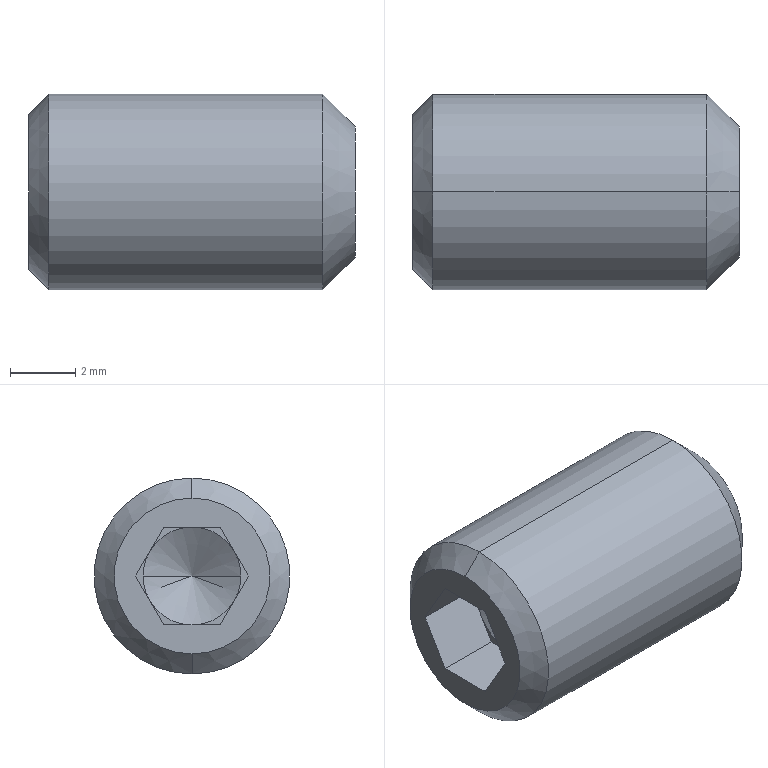Part | SolidWorks | features BaseBody 1 | 1 solid | 22 faces | box 10 x 6 x 6 mm | volume 253.469 mm3 | plane 14 | cone 6 | cylinder 2 | commonest cylinder face diameters 6 x2
STEP:
#1=CARTESIAN_POINT('',(4.,0.,3.));
#2=VERTEX_POINT('',#1);
#3=CARTESIAN_POINT('',(4.,0.,-3.));
#4=VERTEX_POINT('',#3);
#5=CARTESIAN_POINT('',(4.,0.,0.));
#6=DIRECTION('',(-1.,0.,0.));
#7=DIRECTION('',(0.,0.,1.));
#8=AXIS2_PLACEMENT_3D('',#5,#6,#7);
#9=CIRCLE('',#8,3.);
#10=EDGE_CURVE('',#2,#4,#9,.T.);
#11=ORIENTED_EDGE('',*,*,#10,.T.);
#12=CARTESIAN_POINT('',(-4.387,0.,-3.));
#13=VERTEX_POINT('',#12);
#14=CARTESIAN_POINT('',(5.,0.,-3.));
#15=DIRECTION('',(-1.,0.,0.));
#16=VECTOR('',#15,1000.);
#17=LINE('',#14,#16);
#18=EDGE_CURVE('',#4,#13,#17,.T.);
#19=ORIENTED_EDGE('',*,*,#18,.T.);
#20=CARTESIAN_POINT('',(-4.387,0.,3.));
#21=VERTEX_POINT('',#20);
#22=CARTESIAN_POINT('',(-4.387,0.,0.));
#23=DIRECTION('',(1.,0.,0.));
#24=DIRECTION('',(0.,0.,1.));
#25=AXIS2_PLACEMENT_3D('',#22,#23,#24);
#26=CIRCLE('',#25,3.);
#27=EDGE_CURVE('',#13,#21,#26,.T.);
#28=ORIENTED_EDGE('',*,*,#27,.T.);
#29=CARTESIAN_POINT('',(5.,0.,3.));
#30=DIRECTION('',(-1.,0.,0.));
#31=VECTOR('',#30,1000.);
#32=LINE('',#29,#31);
#33=EDGE_CURVE('',#2,#21,#32,.T.);
#34=ORIENTED_EDGE('',*,*,#33,.F.);
#35=EDGE_LOOP('',(#11,#19,#28,#34));
#36=FACE_OUTER_BOUND('',#35,.T.);
#37=CARTESIAN_POINT('',(5.,0.,0.));
#38=DIRECTION('',(-1.,0.,0.));
#39=DIRECTION('',(0.,0.,1.));
#40=AXIS2_PLACEMENT_3D('',#37,#38,#39);
#41=CYLINDRICAL_SURFACE('',#40,3.);
#42=ADVANCED_FACE('',(#36),#41,.T.);
#43=CARTESIAN_POINT('',(-5.,0.,-2.387));
#44=VERTEX_POINT('',#43);
#45=CARTESIAN_POINT('',(-5.,0.,2.387));
#46=VERTEX_POINT('',#45);
#47=CARTESIAN_POINT('',(-5.,0.,0.));
#48=DIRECTION('',(1.,0.,0.));
#49=DIRECTION('',(0.,0.,-1.));
#50=AXIS2_PLACEMENT_3D('',#47,#48,#49);
#51=CIRCLE('',#50,2.387);
#52=EDGE_CURVE('',#44,#46,#51,.T.);
#53=ORIENTED_EDGE('',*,*,#52,.T.);
#54=CARTESIAN_POINT('',(-4.387,0.,3.));
#55=DIRECTION('',(0.7071,0.,0.7071));
#56=VECTOR('',#55,1000.);
#57=LINE('',#54,#56);
#58=EDGE_CURVE('',#46,#21,#57,.T.);
#59=ORIENTED_EDGE('',*,*,#58,.T.);
#60=ORIENTED_EDGE('',*,*,#27,.F.);
#61=CARTESIAN_POINT('',(-4.387,0.,-3.));
#62=DIRECTION('',(0.7071,0.,-0.7071));
#63=VECTOR('',#62,1000.);
#64=LINE('',#61,#63);
#65=EDGE_CURVE('',#44,#13,#64,.T.);
#66=ORIENTED_EDGE('',*,*,#65,.F.);
#67=EDGE_LOOP('',(#53,#59,#60,#66));
#68=FACE_OUTER_BOUND('',#67,.T.);
#69=CARTESIAN_POINT('',(-4.387,0.,0.));
#70=DIRECTION('',(1.,0.,0.));
#71=DIRECTION('',(0.,0.,-1.));
#72=AXIS2_PLACEMENT_3D('',#69,#70,#71);
#73=CONICAL_SURFACE('',#72,3.,0.7854);
#74=ADVANCED_FACE('',(#68),#73,.T.);
#75=CARTESIAN_POINT('',(5.,0.,2.));
#76=VERTEX_POINT('',#75);
#77=CARTESIAN_POINT('',(5.,0.,-2.));
#78=VERTEX_POINT('',#77);
#79=CARTESIAN_POINT('',(5.,0.,0.));
#80=DIRECTION('',(-1.,0.,0.));
#81=DIRECTION('',(0.,0.,1.));
#82=AXIS2_PLACEMENT_3D('',#79,#80,#81);
#83=CIRCLE('',#82,2.);
#84=EDGE_CURVE('',#76,#78,#83,.T.);
#85=ORIENTED_EDGE('',*,*,#84,.T.);
#86=CARTESIAN_POINT('',(4.,0.,-3.));
#87=DIRECTION('',(-0.7071,0.,-0.7071));
#88=VECTOR('',#87,1000.);
#89=LINE('',#86,#88);
#90=EDGE_CURVE('',#78,#4,#89,.T.);
#91=ORIENTED_EDGE('',*,*,#90,.T.);
#92=ORIENTED_EDGE('',*,*,#10,.F.);
#93=CARTESIAN_POINT('',(4.,0.,3.));
#94=DIRECTION('',(-0.7071,0.,0.7071));
#95=VECTOR('',#94,1000.);
#96=LINE('',#93,#95);
#97=EDGE_CURVE('',#76,#2,#96,.T.);
#98=ORIENTED_EDGE('',*,*,#97,.F.);
#99=EDGE_LOOP('',(#85,#91,#92,#98));
#100=FACE_OUTER_BOUND('',#99,.T.);
#101=CARTESIAN_POINT('',(4.,0.,0.));
#102=DIRECTION('',(-1.,0.,0.));
#103=DIRECTION('',(0.,0.,1.));
#104=AXIS2_PLACEMENT_3D('',#101,#102,#103);
#105=CONICAL_SURFACE('',#104,3.,0.7854);
#106=ADVANCED_FACE('',(#100),#105,.T.);
#107=CARTESIAN_POINT('',(-2.15,0.,0.));
#108=VERTEX_POINT('',#107);
#109=CARTESIAN_POINT('',(-3.,-1.5,0.));
#110=VERTEX_POINT('',#109);
#111=CARTESIAN_POINT('',(-3.,-1.5,0.));
#112=DIRECTION('',(-0.493,-0.87,0.));
#113=VECTOR('',#112,1000.);
#114=LINE('',#111,#113);
#115=EDGE_CURVE('',#108,#110,#114,.T.);
#116=ORIENTED_EDGE('',*,*,#115,.F.);
#117=CARTESIAN_POINT('',(-3.,1.5,0.));
#118=VERTEX_POINT('',#117);
#119=CARTESIAN_POINT('',(-3.,1.5,0.));
#120=DIRECTION('',(-0.493,0.87,0.));
#121=VECTOR('',#120,1000.);
#122=LINE('',#119,#121);
#123=EDGE_CURVE('',#108,#118,#122,.T.);
#124=ORIENTED_EDGE('',*,*,#123,.T.);
#125=CARTESIAN_POINT('',(-3.,1.299,-0.75));
#126=VERTEX_POINT('',#125);
#127=CARTESIAN_POINT('',(-3.,0.,0.));
#128=DIRECTION('',(-1.,0.,0.));
#129=DIRECTION('',(0.,-1.,0.));
#130=AXIS2_PLACEMENT_3D('',#127,#128,#129);
#131=CIRCLE('',#130,1.5);
#132=EDGE_CURVE('',#118,#126,#131,.T.);
#133=ORIENTED_EDGE('',*,*,#132,.T.);
#134=CARTESIAN_POINT('',(-3.,0.,-1.5));
#135=VERTEX_POINT('',#134);
#136=CARTESIAN_POINT('',(-3.,0.,0.));
#137=DIRECTION('',(1.,0.,0.));
#138=DIRECTION('',(0.,-1.,0.));
#139=AXIS2_PLACEMENT_3D('',#136,#137,#138);
#140=CIRCLE('',#139,1.5);
#141=EDGE_CURVE('',#135,#126,#140,.T.);
#142=ORIENTED_EDGE('',*,*,#141,.F.);
#143=CARTESIAN_POINT('',(-3.,-1.299,-0.75));
#144=VERTEX_POINT('',#143);
#145=CARTESIAN_POINT('',(-3.,0.,0.));
#146=DIRECTION('',(1.,0.,0.));
#147=DIRECTION('',(0.,-1.,0.));
#148=AXIS2_PLACEMENT_3D('',#145,#146,#147);
#149=CIRCLE('',#148,1.5);
#150=EDGE_CURVE('',#144,#135,#149,.T.);
#151=ORIENTED_EDGE('',*,*,#150,.F.);
#152=CARTESIAN_POINT('',(-3.,0.,0.));
#153=DIRECTION('',(1.,0.,0.));
#154=DIRECTION('',(0.,-1.,0.));
#155=AXIS2_PLACEMENT_3D('',#152,#153,#154);
#156=CIRCLE('',#155,1.5);
#157=EDGE_CURVE('',#110,#144,#156,.T.);
#158=ORIENTED_EDGE('',*,*,#157,.F.);
#159=EDGE_LOOP('',(#116,#124,#133,#142,#151,#158));
#160=FACE_OUTER_BOUND('',#159,.T.);
#161=CARTESIAN_POINT('',(-3.,0.,0.));
#162=DIRECTION('',(-1.,0.,0.));
#163=DIRECTION('',(0.,-1.,0.));
#164=AXIS2_PLACEMENT_3D('',#161,#162,#163);
#165=CONICAL_SURFACE('',#164,1.5,1.055);
#166=ADVANCED_FACE('',(#160),#165,.F.);
#167=ORIENTED_EDGE('',*,*,#18,.F.);
#168=CARTESIAN_POINT('',(4.,0.,0.));
#169=DIRECTION('',(-1.,0.,0.));
#170=DIRECTION('',(0.,0.,1.));
#171=AXIS2_PLACEMENT_3D('',#168,#169,#170);
#172=CIRCLE('',#171,3.);
#173=EDGE_CURVE('',#4,#2,#172,.T.);
#174=ORIENTED_EDGE('',*,*,#173,.T.);
#175=ORIENTED_EDGE('',*,*,#33,.T.);
#176=CARTESIAN_POINT('',(-4.387,0.,0.));
#177=DIRECTION('',(1.,0.,0.));
#178=DIRECTION('',(0.,0.,1.));
#179=AXIS2_PLACEMENT_3D('',#176,#177,#178);
#180=CIRCLE('',#179,3.);
#181=EDGE_CURVE('',#21,#13,#180,.T.);
#182=ORIENTED_EDGE('',*,*,#181,.T.);
#183=EDGE_LOOP('',(#167,#174,#175,#182));
#184=FACE_OUTER_BOUND('',#183,.T.);
#185=CARTESIAN_POINT('',(5.,0.,0.));
#186=DIRECTION('',(-1.,0.,0.));
#187=DIRECTION('',(0.,0.,1.));
#188=AXIS2_PLACEMENT_3D('',#185,#186,#187);
#189=CYLINDRICAL_SURFACE('',#188,3.);
#190=ADVANCED_FACE('',(#184),#189,.T.);
#191=ORIENTED_EDGE('',*,*,#58,.F.);
#192=CARTESIAN_POINT('',(-5.,0.,0.));
#193=DIRECTION('',(1.,0.,0.));
#194=DIRECTION('',(0.,0.,-1.));
#195=AXIS2_PLACEMENT_3D('',#192,#193,#194);
#196=CIRCLE('',#195,2.387);
#197=EDGE_CURVE('',#46,#44,#196,.T.);
#198=ORIENTED_EDGE('',*,*,#197,.T.);
#199=ORIENTED_EDGE('',*,*,#65,.T.);
#200=ORIENTED_EDGE('',*,*,#181,.F.);
#201=EDGE_LOOP('',(#191,#198,#199,#200));
#202=FACE_OUTER_BOUND('',#201,.T.);
#203=CARTESIAN_POINT('',(-4.387,0.,0.));
#204=DIRECTION('',(1.,0.,0.));
#205=DIRECTION('',(0.,0.,-1.));
#206=AXIS2_PLACEMENT_3D('',#203,#204,#205);
#207=CONICAL_SURFACE('',#206,3.,0.7854);
#208=ADVANCED_FACE('',(#202),#207,.T.);
#209=ORIENTED_EDGE('',*,*,#90,.F.);
#210=CARTESIAN_POINT('',(5.,0.,0.));
#211=DIRECTION('',(-1.,0.,0.));
#212=DIRECTION('',(0.,0.,1.));
#213=AXIS2_PLACEMENT_3D('',#210,#211,#212);
#214=CIRCLE('',#213,2.);
#215=EDGE_CURVE('',#78,#76,#214,.T.);
#216=ORIENTED_EDGE('',*,*,#215,.T.);
#217=ORIENTED_EDGE('',*,*,#97,.T.);
#218=ORIENTED_EDGE('',*,*,#173,.F.);
#219=EDGE_LOOP('',(#209,#216,#217,#218));
#220=FACE_OUTER_BOUND('',#219,.T.);
#221=CARTESIAN_POINT('',(4.,0.,0.));
#222=DIRECTION('',(-1.,0.,0.));
#223=DIRECTION('',(0.,0.,1.));
#224=AXIS2_PLACEMENT_3D('',#221,#222,#223);
#225=CONICAL_SURFACE('',#224,3.,0.7854);
#226=ADVANCED_FACE('',(#220),#225,.T.);
#227=CARTESIAN_POINT('',(-5.,-0.866,1.5));
#228=VERTEX_POINT('',#227);
#229=CARTESIAN_POINT('',(-5.,0.866,1.5));
#230=VERTEX_POINT('',#229);
#231=CARTESIAN_POINT('',(-5.,0.866,1.5));
#232=DIRECTION('',(0.,1.,0.));
#233=VECTOR('',#232,1000.);
#234=LINE('',#231,#233);
#235=EDGE_CURVE('',#228,#230,#234,.T.);
#236=ORIENTED_EDGE('',*,*,#235,.F.);
#237=CARTESIAN_POINT('',(-5.,-1.732,0.));
#238=VERTEX_POINT('',#237);
#239=CARTESIAN_POINT('',(-5.,-0.866,1.5));
#240=DIRECTION('',(0.,0.5,0.866));
#241=VECTOR('',#240,1000.);
#242=LINE('',#239,#241);
#243=EDGE_CURVE('',#238,#228,#242,.T.);
#244=ORIENTED_EDGE('',*,*,#243,.F.);
#245=CARTESIAN_POINT('',(-5.,-0.866,-1.5));
#246=VERTEX_POINT('',#245);
#247=CARTESIAN_POINT('',(-5.,-1.732,0.));
#248=DIRECTION('',(0.,-0.5,0.866));
#249=VECTOR('',#248,1000.);
#250=LINE('',#247,#249);
#251=EDGE_CURVE('',#246,#238,#250,.T.);
#252=ORIENTED_EDGE('',*,*,#251,.F.);
#253=CARTESIAN_POINT('',(-5.,0.866,-1.5));
#254=VERTEX_POINT('',#253);
#255=CARTESIAN_POINT('',(-5.,-0.866,-1.5));
#256=DIRECTION('',(0.,-1.,0.));
#257=VECTOR('',#256,1000.);
#258=LINE('',#255,#257);
#259=EDGE_CURVE('',#254,#246,#258,.T.);
#260=ORIENTED_EDGE('',*,*,#259,.F.);
#261=CARTESIAN_POINT('',(-5.,1.732,0.));
#262=VERTEX_POINT('',#261);
#263=CARTESIAN_POINT('',(-5.,0.866,-1.5));
#264=DIRECTION('',(0.,-0.5,-0.866));
#265=VECTOR('',#264,1000.);
#266=LINE('',#263,#265);
#267=EDGE_CURVE('',#262,#254,#266,.T.);
#268=ORIENTED_EDGE('',*,*,#267,.F.);
#269=CARTESIAN_POINT('',(-5.,0.866,1.5));
#270=DIRECTION('',(0.,0.5,-0.866));
#271=VECTOR('',#270,1000.);
#272=LINE('',#269,#271);
#273=EDGE_CURVE('',#230,#262,#272,.T.);
#274=ORIENTED_EDGE('',*,*,#273,.F.);
#275=EDGE_LOOP('',(#236,#244,#252,#260,#268,#274));
#276=FACE_BOUND('',#275,.T.);
#277=ORIENTED_EDGE('',*,*,#52,.F.);
#278=ORIENTED_EDGE('',*,*,#197,.F.);
#279=EDGE_LOOP('',(#277,#278));
#280=FACE_OUTER_BOUND('',#279,.T.);
#281=CARTESIAN_POINT('',(-5.,0.,0.));
#282=DIRECTION('',(1.,0.,0.));
#283=DIRECTION('',(0.,0.,-1.));
#284=AXIS2_PLACEMENT_3D('',#281,#282,#283);
#285=PLANE('',#284);
#286=ADVANCED_FACE('',(#276,#280),#285,.F.);
#287=ORIENTED_EDGE('',*,*,#84,.F.);
#288=ORIENTED_EDGE('',*,*,#215,.F.);
#289=EDGE_LOOP('',(#287,#288));
#290=FACE_OUTER_BOUND('',#289,.T.);
#291=CARTESIAN_POINT('',(5.,2.,0.));
#292=DIRECTION('',(-1.,0.,0.));
#293=DIRECTION('',(0.,0.,1.));
#294=AXIS2_PLACEMENT_3D('',#291,#292,#293);
#295=PLANE('',#294);
#296=ADVANCED_FACE('',(#290),#295,.F.);
#297=CARTESIAN_POINT('',(-3.,1.299,0.75));
#298=VERTEX_POINT('',#297);
#299=CARTESIAN_POINT('',(-3.,0.866,1.5));
#300=VERTEX_POINT('',#299);
#301=CARTESIAN_POINT('',(-3.,1.732,0.));
#302=DIRECTION('',(0.,-0.5,0.866));
#303=VECTOR('',#302,1000.);
#304=LINE('',#301,#303);
#305=EDGE_CURVE('',#298,#300,#304,.T.);
#306=ORIENTED_EDGE('',*,*,#305,.T.);
#307=CARTESIAN_POINT('',(-3.,0.866,1.5));
#308=DIRECTION('',(-1.,0.,0.));
#309=VECTOR('',#308,1000.);
#310=LINE('',#307,#309);
#311=EDGE_CURVE('',#300,#230,#310,.T.);
#312=ORIENTED_EDGE('',*,*,#311,.T.);
#313=ORIENTED_EDGE('',*,*,#273,.T.);
#314=CARTESIAN_POINT('',(-3.,1.732,0.));
#315=VERTEX_POINT('',#314);
#316=CARTESIAN_POINT('',(-3.,1.732,0.));
#317=DIRECTION('',(1.,0.,0.));
#318=VECTOR('',#317,1000.);
#319=LINE('',#316,#318);
#320=EDGE_CURVE('',#262,#315,#319,.T.);
#321=ORIENTED_EDGE('',*,*,#320,.T.);
#322=CARTESIAN_POINT('',(-3.,1.732,0.));
#323=DIRECTION('',(0.,-0.5,0.866));
#324=VECTOR('',#323,1000.);
#325=LINE('',#322,#324);
#326=EDGE_CURVE('',#315,#298,#325,.T.);
#327=ORIENTED_EDGE('',*,*,#326,.T.);
#328=EDGE_LOOP('',(#306,#312,#313,#321,#327));
#329=FACE_OUTER_BOUND('',#328,.T.);
#330=CARTESIAN_POINT('',(-3.,1.732,0.));
#331=DIRECTION('',(0.,-0.866,-0.5));
#332=DIRECTION('',(0.,0.5,-0.866));
#333=AXIS2_PLACEMENT_3D('',#330,#331,#332);
#334=PLANE('',#333);
#335=ADVANCED_FACE('',(#329),#334,.T.);
#336=CARTESIAN_POINT('',(-3.,0.,1.5));
#337=VERTEX_POINT('',#336);
#338=CARTESIAN_POINT('',(-3.,-0.866,1.5));
#339=VERTEX_POINT('',#338);
#340=CARTESIAN_POINT('',(-3.,0.866,1.5));
#341=DIRECTION('',(0.,-1.,0.));
#342=VECTOR('',#341,1000.);
#343=LINE('',#340,#342);
#344=EDGE_CURVE('',#337,#339,#343,.T.);
#345=ORIENTED_EDGE('',*,*,#344,.T.);
#346=CARTESIAN_POINT('',(-3.,-0.866,1.5));
#347=DIRECTION('',(-1.,0.,0.));
#348=VECTOR('',#347,1000.);
#349=LINE('',#346,#348);
#350=EDGE_CURVE('',#339,#228,#349,.T.);
#351=ORIENTED_EDGE('',*,*,#350,.T.);
#352=ORIENTED_EDGE('',*,*,#235,.T.);
#353=ORIENTED_EDGE('',*,*,#311,.F.);
#354=CARTESIAN_POINT('',(-3.,0.866,1.5));
#355=DIRECTION('',(0.,-1.,0.));
#356=VECTOR('',#355,1000.);
#357=LINE('',#354,#356);
#358=EDGE_CURVE('',#300,#337,#357,.T.);
#359=ORIENTED_EDGE('',*,*,#358,.T.);
#360=EDGE_LOOP('',(#345,#351,#352,#353,#359));
#361=FACE_OUTER_BOUND('',#360,.T.);
#362=CARTESIAN_POINT('',(-3.,0.866,1.5));
#363=DIRECTION('',(0.,0.,-1.));
#364=DIRECTION('',(-1.,0.,0.));
#365=AXIS2_PLACEMENT_3D('',#362,#363,#364);
#366=PLANE('',#365);
#367=ADVANCED_FACE('',(#361),#366,.T.);
#368=ORIENTED_EDGE('',*,*,#358,.F.);
#369=ORIENTED_EDGE('',*,*,#305,.F.);
#370=CARTESIAN_POINT('',(-3.,0.,0.));
#371=DIRECTION('',(-1.,0.,0.));
#372=DIRECTION('',(0.,-1.,0.));
#373=AXIS2_PLACEMENT_3D('',#370,#371,#372);
#374=CIRCLE('',#373,1.5);
#375=EDGE_CURVE('',#337,#298,#374,.T.);
#376=ORIENTED_EDGE('',*,*,#375,.F.);
#377=EDGE_LOOP('',(#368,#369,#376));
#378=FACE_OUTER_BOUND('',#377,.T.);
#379=CARTESIAN_POINT('',(-3.,0.,0.));
#380=DIRECTION('',(1.,0.,0.));
#381=DIRECTION('',(0.,0.,-1.));
#382=AXIS2_PLACEMENT_3D('',#379,#380,#381);
#383=PLANE('',#382);
#384=ADVANCED_FACE('',(#378),#383,.F.);
#385=ORIENTED_EDGE('',*,*,#326,.F.);
#386=CARTESIAN_POINT('',(-3.,1.299,-0.75));
#387=DIRECTION('',(0.,0.5,0.866));
#388=VECTOR('',#387,1000.);
#389=LINE('',#386,#388);
#390=EDGE_CURVE('',#126,#315,#389,.T.);
#391=ORIENTED_EDGE('',*,*,#390,.F.);
#392=ORIENTED_EDGE('',*,*,#132,.F.);
#393=CARTESIAN_POINT('',(-3.,0.,0.));
#394=DIRECTION('',(-1.,0.,0.));
#395=DIRECTION('',(0.,-1.,0.));
#396=AXIS2_PLACEMENT_3D('',#393,#394,#395);
#397=CIRCLE('',#396,1.5);
#398=EDGE_CURVE('',#298,#118,#397,.T.);
#399=ORIENTED_EDGE('',*,*,#398,.F.);
#400=EDGE_LOOP('',(#385,#391,#392,#399));
#401=FACE_OUTER_BOUND('',#400,.T.);
#402=CARTESIAN_POINT('',(-3.,0.,0.));
#403=DIRECTION('',(1.,0.,0.));
#404=DIRECTION('',(0.,0.,-1.));
#405=AXIS2_PLACEMENT_3D('',#402,#403,#404);
#406=PLANE('',#405);
#407=ADVANCED_FACE('',(#401),#406,.F.);
#408=ORIENTED_EDGE('',*,*,#390,.T.);
#409=ORIENTED_EDGE('',*,*,#320,.F.);
#410=ORIENTED_EDGE('',*,*,#267,.T.);
#411=CARTESIAN_POINT('',(-3.,0.866,-1.5));
#412=VERTEX_POINT('',#411);
#413=CARTESIAN_POINT('',(-3.,0.866,-1.5));
#414=DIRECTION('',(1.,0.,0.));
#415=VECTOR('',#414,1000.);
#416=LINE('',#413,#415);
#417=EDGE_CURVE('',#254,#412,#416,.T.);
#418=ORIENTED_EDGE('',*,*,#417,.T.);
#419=CARTESIAN_POINT('',(-3.,0.866,-1.5));
#420=DIRECTION('',(0.,0.5,0.866));
#421=VECTOR('',#420,1000.);
#422=LINE('',#419,#421);
#423=EDGE_CURVE('',#412,#126,#422,.T.);
#424=ORIENTED_EDGE('',*,*,#423,.T.);
#425=EDGE_LOOP('',(#408,#409,#410,#418,#424));
#426=FACE_OUTER_BOUND('',#425,.T.);
#427=CARTESIAN_POINT('',(-3.,0.866,-1.5));
#428=DIRECTION('',(0.,-0.866,0.5));
#429=DIRECTION('',(0.,-0.5,-0.866));
#430=AXIS2_PLACEMENT_3D('',#427,#428,#429);
#431=PLANE('',#430);
#432=ADVANCED_FACE('',(#426),#431,.T.);
#433=CARTESIAN_POINT('',(-3.,-1.299,0.75));
#434=VERTEX_POINT('',#433);
#435=CARTESIAN_POINT('',(-3.,-1.732,0.));
#436=VERTEX_POINT('',#435);
#437=CARTESIAN_POINT('',(-3.,-0.866,1.5));
#438=DIRECTION('',(0.,-0.5,-0.866));
#439=VECTOR('',#438,1000.);
#440=LINE('',#437,#439);
#441=EDGE_CURVE('',#434,#436,#440,.T.);
#442=ORIENTED_EDGE('',*,*,#441,.T.);
#443=CARTESIAN_POINT('',(-3.,-1.732,0.));
#444=DIRECTION('',(-1.,0.,0.));
#445=VECTOR('',#444,1000.);
#446=LINE('',#443,#445);
#447=EDGE_CURVE('',#436,#238,#446,.T.);
#448=ORIENTED_EDGE('',*,*,#447,.T.);
#449=ORIENTED_EDGE('',*,*,#243,.T.);
#450=ORIENTED_EDGE('',*,*,#350,.F.);
#451=CARTESIAN_POINT('',(-3.,-0.866,1.5));
#452=DIRECTION('',(0.,-0.5,-0.866));
#453=VECTOR('',#452,1000.);
#454=LINE('',#451,#453);
#455=EDGE_CURVE('',#339,#434,#454,.T.);
#456=ORIENTED_EDGE('',*,*,#455,.T.);
#457=EDGE_LOOP('',(#442,#448,#449,#450,#456));
#458=FACE_OUTER_BOUND('',#457,.T.);
#459=CARTESIAN_POINT('',(-3.,-0.866,1.5));
#460=DIRECTION('',(0.,0.866,-0.5));
#461=DIRECTION('',(0.,0.5,0.866));
#462=AXIS2_PLACEMENT_3D('',#459,#460,#461);
#463=PLANE('',#462);
#464=ADVANCED_FACE('',(#458),#463,.T.);
#465=ORIENTED_EDGE('',*,*,#455,.F.);
#466=ORIENTED_EDGE('',*,*,#344,.F.);
#467=CARTESIAN_POINT('',(-3.,0.,0.));
#468=DIRECTION('',(-1.,0.,0.));
#469=DIRECTION('',(0.,-1.,0.));
#470=AXIS2_PLACEMENT_3D('',#467,#468,#469);
#471=CIRCLE('',#470,1.5);
#472=EDGE_CURVE('',#434,#337,#471,.T.);
#473=ORIENTED_EDGE('',*,*,#472,.F.);
#474=EDGE_LOOP('',(#465,#466,#473));
#475=FACE_OUTER_BOUND('',#474,.T.);
#476=CARTESIAN_POINT('',(-3.,0.,0.));
#477=DIRECTION('',(1.,0.,0.));
#478=DIRECTION('',(0.,0.,-1.));
#479=AXIS2_PLACEMENT_3D('',#476,#477,#478);
#480=PLANE('',#479);
#481=ADVANCED_FACE('',(#475),#480,.F.);
#482=ORIENTED_EDGE('',*,*,#123,.F.);
#483=ORIENTED_EDGE('',*,*,#115,.T.);
#484=CARTESIAN_POINT('',(-3.,0.,0.));
#485=DIRECTION('',(1.,0.,0.));
#486=DIRECTION('',(0.,-1.,0.));
#487=AXIS2_PLACEMENT_3D('',#484,#485,#486);
#488=CIRCLE('',#487,1.5);
#489=EDGE_CURVE('',#434,#110,#488,.T.);
#490=ORIENTED_EDGE('',*,*,#489,.F.);
#491=ORIENTED_EDGE('',*,*,#472,.T.);
#492=ORIENTED_EDGE('',*,*,#375,.T.);
#493=ORIENTED_EDGE('',*,*,#398,.T.);
#494=EDGE_LOOP('',(#482,#483,#490,#491,#492,#493));
#495=FACE_OUTER_BOUND('',#494,.T.);
#496=CARTESIAN_POINT('',(-3.,0.,0.));
#497=DIRECTION('',(-1.,0.,0.));
#498=DIRECTION('',(0.,-1.,0.));
#499=AXIS2_PLACEMENT_3D('',#496,#497,#498);
#500=CONICAL_SURFACE('',#499,1.5,1.055);
#501=ADVANCED_FACE('',(#495),#500,.F.);
#502=ORIENTED_EDGE('',*,*,#423,.F.);
#503=CARTESIAN_POINT('',(-3.,0.,-1.5));
#504=DIRECTION('',(0.,1.,0.));
#505=VECTOR('',#504,1000.);
#506=LINE('',#503,#505);
#507=EDGE_CURVE('',#135,#412,#506,.T.);
#508=ORIENTED_EDGE('',*,*,#507,.F.);
#509=ORIENTED_EDGE('',*,*,#141,.T.);
#510=EDGE_LOOP('',(#502,#508,#509));
#511=FACE_OUTER_BOUND('',#510,.T.);
#512=CARTESIAN_POINT('',(-3.,0.,0.));
#513=DIRECTION('',(1.,0.,0.));
#514=DIRECTION('',(0.,0.,-1.));
#515=AXIS2_PLACEMENT_3D('',#512,#513,#514);
#516=PLANE('',#515);
#517=ADVANCED_FACE('',(#511),#516,.F.);
#518=ORIENTED_EDGE('',*,*,#507,.T.);
#519=ORIENTED_EDGE('',*,*,#417,.F.);
#520=ORIENTED_EDGE('',*,*,#259,.T.);
#521=CARTESIAN_POINT('',(-3.,-0.866,-1.5));
#522=VERTEX_POINT('',#521);
#523=CARTESIAN_POINT('',(-3.,-0.866,-1.5));
#524=DIRECTION('',(1.,0.,0.));
#525=VECTOR('',#524,1000.);
#526=LINE('',#523,#525);
#527=EDGE_CURVE('',#246,#522,#526,.T.);
#528=ORIENTED_EDGE('',*,*,#527,.T.);
#529=CARTESIAN_POINT('',(-3.,-0.866,-1.5));
#530=DIRECTION('',(0.,1.,0.));
#531=VECTOR('',#530,1000.);
#532=LINE('',#529,#531);
#533=EDGE_CURVE('',#522,#135,#532,.T.);
#534=ORIENTED_EDGE('',*,*,#533,.T.);
#535=EDGE_LOOP('',(#518,#519,#520,#528,#534));
#536=FACE_OUTER_BOUND('',#535,.T.);
#537=CARTESIAN_POINT('',(-3.,-0.866,-1.5));
#538=DIRECTION('',(0.,0.,1.));
#539=DIRECTION('',(1.,0.,0.));
#540=AXIS2_PLACEMENT_3D('',#537,#538,#539);
#541=PLANE('',#540);
#542=ADVANCED_FACE('',(#536),#541,.T.);
#543=CARTESIAN_POINT('',(-3.,-1.732,0.));
#544=DIRECTION('',(0.,0.5,-0.866));
#545=VECTOR('',#544,1000.);
#546=LINE('',#543,#545);
#547=EDGE_CURVE('',#144,#522,#546,.T.);
#548=ORIENTED_EDGE('',*,*,#547,.T.);
#549=ORIENTED_EDGE('',*,*,#527,.F.);
#550=ORIENTED_EDGE('',*,*,#251,.T.);
#551=ORIENTED_EDGE('',*,*,#447,.F.);
#552=CARTESIAN_POINT('',(-3.,-1.732,0.));
#553=DIRECTION('',(0.,0.5,-0.866));
#554=VECTOR('',#553,1000.);
#555=LINE('',#552,#554);
#556=EDGE_CURVE('',#436,#144,#555,.T.);
#557=ORIENTED_EDGE('',*,*,#556,.T.);
#558=EDGE_LOOP('',(#548,#549,#550,#551,#557));
#559=FACE_OUTER_BOUND('',#558,.T.);
#560=CARTESIAN_POINT('',(-3.,-1.732,0.));
#561=DIRECTION('',(0.,0.866,0.5));
#562=DIRECTION('',(0.,-0.5,0.866));
#563=AXIS2_PLACEMENT_3D('',#560,#561,#562);
#564=PLANE('',#563);
#565=ADVANCED_FACE('',(#559),#564,.T.);
#566=ORIENTED_EDGE('',*,*,#556,.F.);
#567=ORIENTED_EDGE('',*,*,#441,.F.);
#568=ORIENTED_EDGE('',*,*,#489,.T.);
#569=ORIENTED_EDGE('',*,*,#157,.T.);
#570=EDGE_LOOP('',(#566,#567,#568,#569));
#571=FACE_OUTER_BOUND('',#570,.T.);
#572=CARTESIAN_POINT('',(-3.,0.,0.));
#573=DIRECTION('',(1.,0.,0.));
#574=DIRECTION('',(0.,0.,-1.));
#575=AXIS2_PLACEMENT_3D('',#572,#573,#574);
#576=PLANE('',#575);
#577=ADVANCED_FACE('',(#571),#576,.F.);
#578=ORIENTED_EDGE('',*,*,#533,.F.);
#579=ORIENTED_EDGE('',*,*,#547,.F.);
#580=ORIENTED_EDGE('',*,*,#150,.T.);
#581=EDGE_LOOP('',(#578,#579,#580));
#582=FACE_OUTER_BOUND('',#581,.T.);
#583=CARTESIAN_POINT('',(-3.,0.,0.));
#584=DIRECTION('',(1.,0.,0.));
#585=DIRECTION('',(0.,0.,-1.));
#586=AXIS2_PLACEMENT_3D('',#583,#584,#585);
#587=PLANE('',#586);
#588=ADVANCED_FACE('',(#582),#587,.F.);
#589=CLOSED_SHELL('',(#42,#74,#106,#166,#190,#208,#226,#286,#296,#335,#367,#384,#407,#432,#464,#481,#501,#517,#542,#565,#577,#588));
#590=MANIFOLD_SOLID_BREP('',#589);
#591=CARTESIAN_POINT('',(0.,0.,0.));
#592=DIRECTION('',(0.,0.,1.));
#593=DIRECTION('',(1.,0.,0.));
#594=AXIS2_PLACEMENT_3D('',#591,#592,#593);
#595=(LENGTH_UNIT()NAMED_UNIT(*)SI_UNIT(.MILLI.,.METRE.));
#596=UNCERTAINTY_MEASURE_WITH_UNIT(LENGTH_MEASURE(0.00001),#595,'','');
#597=(NAMED_UNIT(*)PLANE_ANGLE_UNIT()SI_UNIT($,.RADIAN.));
#598=(NAMED_UNIT(*)SI_UNIT($,.STERADIAN.)SOLID_ANGLE_UNIT());
#599=(GEOMETRIC_REPRESENTATION_CONTEXT(3)GLOBAL_UNCERTAINTY_ASSIGNED_CONTEXT((#596))GLOBAL_UNIT_ASSIGNED_CONTEXT((#595,#597,#598))REPRESENTATION_CONTEXT('',''));
#600=ADVANCED_BREP_SHAPE_REPRESENTATION('',(#590,#594),#599);